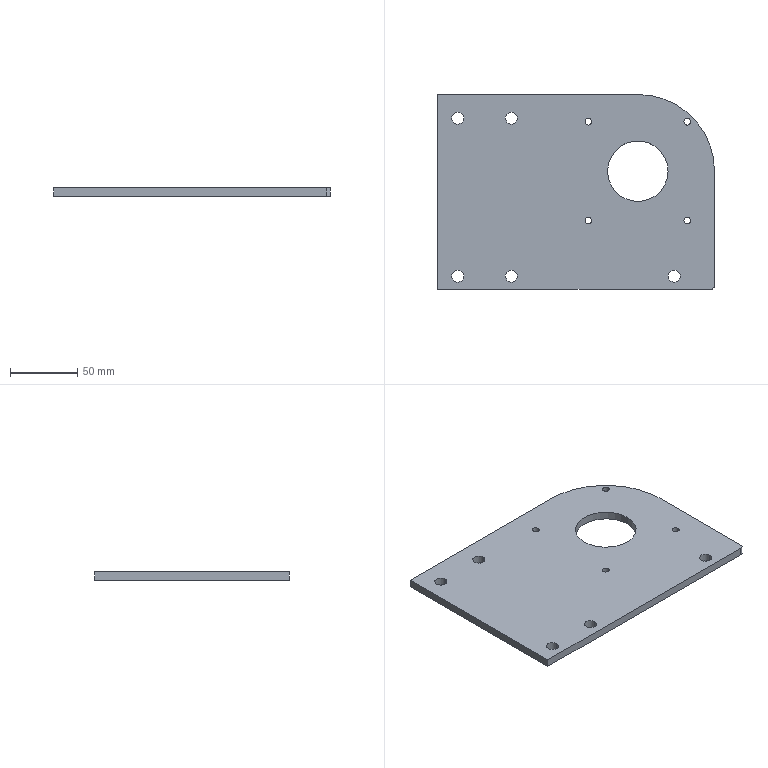Part | SolidWorks | features ICE 6, Fillet 5, HoleWzd 2, CirPattern 1, Extrusion 1 | 1 solid | 28 faces | box 206 x 145 x 6 mm | volume 163103 mm3 | cylinder 22 | plane 6 | commonest cylinder face diameters 9 x10 5 x8 45 x2 6 x1 114 x1
STEP:
#1=CARTESIAN_POINT('',(68.5,-62.5,0.));
#2=VERTEX_POINT('',#1);
#3=CARTESIAN_POINT('',(77.5,-62.5,0.));
#4=VERTEX_POINT('',#3);
#5=CARTESIAN_POINT('',(73.,-62.5,0.));
#6=DIRECTION('',(0.,0.,1.));
#7=DIRECTION('',(1.,0.,0.));
#8=AXIS2_PLACEMENT_3D('',#5,#6,#7);
#9=CIRCLE('',#8,4.5);
#10=EDGE_CURVE('',#2,#4,#9,.T.);
#11=ORIENTED_EDGE('',*,*,#10,.F.);
#12=CARTESIAN_POINT('',(68.5,-62.5,6.));
#13=VERTEX_POINT('',#12);
#14=CARTESIAN_POINT('',(68.5,-62.5,0.));
#15=DIRECTION('',(0.,0.,1.));
#16=VECTOR('',#15,1000.);
#17=LINE('',#14,#16);
#18=EDGE_CURVE('',#2,#13,#17,.T.);
#19=ORIENTED_EDGE('',*,*,#18,.T.);
#20=CARTESIAN_POINT('',(77.5,-62.5,6.));
#21=VERTEX_POINT('',#20);
#22=CARTESIAN_POINT('',(73.,-62.5,6.));
#23=DIRECTION('',(0.,0.,1.));
#24=DIRECTION('',(1.,0.,0.));
#25=AXIS2_PLACEMENT_3D('',#22,#23,#24);
#26=CIRCLE('',#25,4.5);
#27=EDGE_CURVE('',#13,#21,#26,.T.);
#28=ORIENTED_EDGE('',*,*,#27,.T.);
#29=CARTESIAN_POINT('',(77.5,-62.5,0.));
#30=DIRECTION('',(0.,0.,1.));
#31=VECTOR('',#30,1000.);
#32=LINE('',#29,#31);
#33=EDGE_CURVE('',#4,#21,#32,.T.);
#34=ORIENTED_EDGE('',*,*,#33,.F.);
#35=EDGE_LOOP('',(#11,#19,#28,#34));
#36=FACE_OUTER_BOUND('',#35,.T.);
#37=CARTESIAN_POINT('',(73.,-62.5,0.));
#38=DIRECTION('',(0.,0.,1.));
#39=DIRECTION('',(1.,0.,0.));
#40=AXIS2_PLACEMENT_3D('',#37,#38,#39);
#41=CYLINDRICAL_SURFACE('',#40,4.5);
#42=ADVANCED_FACE('',(#36),#41,.F.);
#43=CARTESIAN_POINT('',(80.27,52.27,0.));
#44=VERTEX_POINT('',#43);
#45=CARTESIAN_POINT('',(85.27,52.27,0.));
#46=VERTEX_POINT('',#45);
#47=CARTESIAN_POINT('',(82.77,52.27,0.));
#48=DIRECTION('',(0.,0.,1.));
#49=DIRECTION('',(1.,0.,0.));
#50=AXIS2_PLACEMENT_3D('',#47,#48,#49);
#51=CIRCLE('',#50,2.5);
#52=EDGE_CURVE('',#44,#46,#51,.T.);
#53=ORIENTED_EDGE('',*,*,#52,.F.);
#54=CARTESIAN_POINT('',(80.27,52.27,6.));
#55=VERTEX_POINT('',#54);
#56=CARTESIAN_POINT('',(80.27,52.27,6.));
#57=DIRECTION('',(0.,0.,1.));
#58=VECTOR('',#57,1000.);
#59=LINE('',#56,#58);
#60=EDGE_CURVE('',#44,#55,#59,.T.);
#61=ORIENTED_EDGE('',*,*,#60,.T.);
#62=CARTESIAN_POINT('',(85.27,52.27,6.));
#63=VERTEX_POINT('',#62);
#64=CARTESIAN_POINT('',(82.77,52.27,6.));
#65=DIRECTION('',(0.,0.,1.));
#66=DIRECTION('',(1.,0.,0.));
#67=AXIS2_PLACEMENT_3D('',#64,#65,#66);
#68=CIRCLE('',#67,2.5);
#69=EDGE_CURVE('',#55,#63,#68,.T.);
#70=ORIENTED_EDGE('',*,*,#69,.T.);
#71=CARTESIAN_POINT('',(85.27,52.27,6.));
#72=DIRECTION('',(0.,0.,1.));
#73=VECTOR('',#72,1000.);
#74=LINE('',#71,#73);
#75=EDGE_CURVE('',#46,#63,#74,.T.);
#76=ORIENTED_EDGE('',*,*,#75,.F.);
#77=EDGE_LOOP('',(#53,#61,#70,#76));
#78=FACE_OUTER_BOUND('',#77,.T.);
#79=CARTESIAN_POINT('',(82.77,52.27,6.));
#80=DIRECTION('',(0.,0.,1.));
#81=DIRECTION('',(1.,0.,0.));
#82=AXIS2_PLACEMENT_3D('',#79,#80,#81);
#83=CYLINDRICAL_SURFACE('',#82,2.5);
#84=ADVANCED_FACE('',(#78),#83,.F.);
#85=CARTESIAN_POINT('',(80.27,-21.27,0.));
#86=VERTEX_POINT('',#85);
#87=CARTESIAN_POINT('',(85.27,-21.27,0.));
#88=VERTEX_POINT('',#87);
#89=CARTESIAN_POINT('',(82.77,-21.27,0.));
#90=DIRECTION('',(0.,0.,1.));
#91=DIRECTION('',(1.,0.,0.));
#92=AXIS2_PLACEMENT_3D('',#89,#90,#91);
#93=CIRCLE('',#92,2.5);
#94=EDGE_CURVE('',#86,#88,#93,.T.);
#95=ORIENTED_EDGE('',*,*,#94,.F.);
#96=CARTESIAN_POINT('',(80.27,-21.27,6.));
#97=VERTEX_POINT('',#96);
#98=CARTESIAN_POINT('',(80.27,-21.27,6.));
#99=DIRECTION('',(0.,0.,1.));
#100=VECTOR('',#99,1000.);
#101=LINE('',#98,#100);
#102=EDGE_CURVE('',#86,#97,#101,.T.);
#103=ORIENTED_EDGE('',*,*,#102,.T.);
#104=CARTESIAN_POINT('',(85.27,-21.27,6.));
#105=VERTEX_POINT('',#104);
#106=CARTESIAN_POINT('',(82.77,-21.27,6.));
#107=DIRECTION('',(0.,0.,1.));
#108=DIRECTION('',(1.,0.,0.));
#109=AXIS2_PLACEMENT_3D('',#106,#107,#108);
#110=CIRCLE('',#109,2.5);
#111=EDGE_CURVE('',#97,#105,#110,.T.);
#112=ORIENTED_EDGE('',*,*,#111,.T.);
#113=CARTESIAN_POINT('',(85.27,-21.27,6.));
#114=DIRECTION('',(0.,0.,1.));
#115=VECTOR('',#114,1000.);
#116=LINE('',#113,#115);
#117=EDGE_CURVE('',#88,#105,#116,.T.);
#118=ORIENTED_EDGE('',*,*,#117,.F.);
#119=EDGE_LOOP('',(#95,#103,#112,#118));
#120=FACE_OUTER_BOUND('',#119,.T.);
#121=CARTESIAN_POINT('',(82.77,-21.27,6.));
#122=DIRECTION('',(0.,0.,1.));
#123=DIRECTION('',(1.,0.,0.));
#124=AXIS2_PLACEMENT_3D('',#121,#122,#123);
#125=CYLINDRICAL_SURFACE('',#124,2.5);
#126=ADVANCED_FACE('',(#120),#125,.F.);
#127=CARTESIAN_POINT('',(6.73,-21.27,0.));
#128=VERTEX_POINT('',#127);
#129=CARTESIAN_POINT('',(11.73,-21.27,0.));
#130=VERTEX_POINT('',#129);
#131=CARTESIAN_POINT('',(9.23,-21.27,0.));
#132=DIRECTION('',(0.,0.,1.));
#133=DIRECTION('',(1.,0.,0.));
#134=AXIS2_PLACEMENT_3D('',#131,#132,#133);
#135=CIRCLE('',#134,2.5);
#136=EDGE_CURVE('',#128,#130,#135,.T.);
#137=ORIENTED_EDGE('',*,*,#136,.F.);
#138=CARTESIAN_POINT('',(6.73,-21.27,6.));
#139=VERTEX_POINT('',#138);
#140=CARTESIAN_POINT('',(6.73,-21.27,6.));
#141=DIRECTION('',(0.,0.,1.));
#142=VECTOR('',#141,1000.);
#143=LINE('',#140,#142);
#144=EDGE_CURVE('',#128,#139,#143,.T.);
#145=ORIENTED_EDGE('',*,*,#144,.T.);
#146=CARTESIAN_POINT('',(11.73,-21.27,6.));
#147=VERTEX_POINT('',#146);
#148=CARTESIAN_POINT('',(9.23,-21.27,6.));
#149=DIRECTION('',(0.,0.,1.));
#150=DIRECTION('',(1.,0.,0.));
#151=AXIS2_PLACEMENT_3D('',#148,#149,#150);
#152=CIRCLE('',#151,2.5);
#153=EDGE_CURVE('',#139,#147,#152,.T.);
#154=ORIENTED_EDGE('',*,*,#153,.T.);
#155=CARTESIAN_POINT('',(11.73,-21.27,6.));
#156=DIRECTION('',(0.,0.,1.));
#157=VECTOR('',#156,1000.);
#158=LINE('',#155,#157);
#159=EDGE_CURVE('',#130,#147,#158,.T.);
#160=ORIENTED_EDGE('',*,*,#159,.F.);
#161=EDGE_LOOP('',(#137,#145,#154,#160));
#162=FACE_OUTER_BOUND('',#161,.T.);
#163=CARTESIAN_POINT('',(9.23,-21.27,6.));
#164=DIRECTION('',(0.,0.,1.));
#165=DIRECTION('',(1.,0.,0.));
#166=AXIS2_PLACEMENT_3D('',#163,#164,#165);
#167=CYLINDRICAL_SURFACE('',#166,2.5);
#168=ADVANCED_FACE('',(#162),#167,.F.);
#169=CARTESIAN_POINT('',(6.73,52.27,0.));
#170=VERTEX_POINT('',#169);
#171=CARTESIAN_POINT('',(11.73,52.27,0.));
#172=VERTEX_POINT('',#171);
#173=CARTESIAN_POINT('',(9.23,52.27,0.));
#174=DIRECTION('',(0.,0.,1.));
#175=DIRECTION('',(1.,0.,0.));
#176=AXIS2_PLACEMENT_3D('',#173,#174,#175);
#177=CIRCLE('',#176,2.5);
#178=EDGE_CURVE('',#170,#172,#177,.T.);
#179=ORIENTED_EDGE('',*,*,#178,.F.);
#180=CARTESIAN_POINT('',(6.73,52.27,6.));
#181=VERTEX_POINT('',#180);
#182=CARTESIAN_POINT('',(6.73,52.27,6.));
#183=DIRECTION('',(0.,0.,1.));
#184=VECTOR('',#183,1000.);
#185=LINE('',#182,#184);
#186=EDGE_CURVE('',#170,#181,#185,.T.);
#187=ORIENTED_EDGE('',*,*,#186,.T.);
#188=CARTESIAN_POINT('',(11.73,52.27,6.));
#189=VERTEX_POINT('',#188);
#190=CARTESIAN_POINT('',(9.23,52.27,6.));
#191=DIRECTION('',(0.,0.,1.));
#192=DIRECTION('',(1.,0.,0.));
#193=AXIS2_PLACEMENT_3D('',#190,#191,#192);
#194=CIRCLE('',#193,2.5);
#195=EDGE_CURVE('',#181,#189,#194,.T.);
#196=ORIENTED_EDGE('',*,*,#195,.T.);
#197=CARTESIAN_POINT('',(11.73,52.27,6.));
#198=DIRECTION('',(0.,0.,1.));
#199=VECTOR('',#198,1000.);
#200=LINE('',#197,#199);
#201=EDGE_CURVE('',#172,#189,#200,.T.);
#202=ORIENTED_EDGE('',*,*,#201,.F.);
#203=EDGE_LOOP('',(#179,#187,#196,#202));
#204=FACE_OUTER_BOUND('',#203,.T.);
#205=CARTESIAN_POINT('',(9.23,52.27,6.));
#206=DIRECTION('',(0.,0.,1.));
#207=DIRECTION('',(1.,0.,0.));
#208=AXIS2_PLACEMENT_3D('',#205,#206,#207);
#209=CYLINDRICAL_SURFACE('',#208,2.5);
#210=ADVANCED_FACE('',(#204),#209,.F.);
#211=CARTESIAN_POINT('',(23.5,15.5,0.));
#212=VERTEX_POINT('',#211);
#213=CARTESIAN_POINT('',(68.5,15.5,0.));
#214=VERTEX_POINT('',#213);
#215=CARTESIAN_POINT('',(46.,15.5,0.));
#216=DIRECTION('',(0.,0.,1.));
#217=DIRECTION('',(1.,0.,0.));
#218=AXIS2_PLACEMENT_3D('',#215,#216,#217);
#219=CIRCLE('',#218,22.5);
#220=EDGE_CURVE('',#212,#214,#219,.T.);
#221=ORIENTED_EDGE('',*,*,#220,.F.);
#222=CARTESIAN_POINT('',(23.5,15.5,6.));
#223=VERTEX_POINT('',#222);
#224=CARTESIAN_POINT('',(23.5,15.5,0.));
#225=DIRECTION('',(0.,0.,1.));
#226=VECTOR('',#225,1000.);
#227=LINE('',#224,#226);
#228=EDGE_CURVE('',#212,#223,#227,.T.);
#229=ORIENTED_EDGE('',*,*,#228,.T.);
#230=CARTESIAN_POINT('',(68.5,15.5,6.));
#231=VERTEX_POINT('',#230);
#232=CARTESIAN_POINT('',(46.,15.5,6.));
#233=DIRECTION('',(0.,0.,1.));
#234=DIRECTION('',(1.,0.,0.));
#235=AXIS2_PLACEMENT_3D('',#232,#233,#234);
#236=CIRCLE('',#235,22.5);
#237=EDGE_CURVE('',#223,#231,#236,.T.);
#238=ORIENTED_EDGE('',*,*,#237,.T.);
#239=CARTESIAN_POINT('',(68.5,15.5,0.));
#240=DIRECTION('',(0.,0.,1.));
#241=VECTOR('',#240,1000.);
#242=LINE('',#239,#241);
#243=EDGE_CURVE('',#214,#231,#242,.T.);
#244=ORIENTED_EDGE('',*,*,#243,.F.);
#245=EDGE_LOOP('',(#221,#229,#238,#244));
#246=FACE_OUTER_BOUND('',#245,.T.);
#247=CARTESIAN_POINT('',(46.,15.5,0.));
#248=DIRECTION('',(0.,0.,1.));
#249=DIRECTION('',(1.,0.,0.));
#250=AXIS2_PLACEMENT_3D('',#247,#248,#249);
#251=CYLINDRICAL_SURFACE('',#250,22.5);
#252=ADVANCED_FACE('',(#246),#251,.F.);
#253=CARTESIAN_POINT('',(-52.5,-62.5,0.));
#254=VERTEX_POINT('',#253);
#255=CARTESIAN_POINT('',(-43.5,-62.5,0.));
#256=VERTEX_POINT('',#255);
#257=CARTESIAN_POINT('',(-48.,-62.5,0.));
#258=DIRECTION('',(0.,0.,1.));
#259=DIRECTION('',(1.,0.,0.));
#260=AXIS2_PLACEMENT_3D('',#257,#258,#259);
#261=CIRCLE('',#260,4.5);
#262=EDGE_CURVE('',#254,#256,#261,.T.);
#263=ORIENTED_EDGE('',*,*,#262,.F.);
#264=CARTESIAN_POINT('',(-52.5,-62.5,6.));
#265=VERTEX_POINT('',#264);
#266=CARTESIAN_POINT('',(-52.5,-62.5,0.));
#267=DIRECTION('',(0.,0.,1.));
#268=VECTOR('',#267,1000.);
#269=LINE('',#266,#268);
#270=EDGE_CURVE('',#254,#265,#269,.T.);
#271=ORIENTED_EDGE('',*,*,#270,.T.);
#272=CARTESIAN_POINT('',(-43.5,-62.5,6.));
#273=VERTEX_POINT('',#272);
#274=CARTESIAN_POINT('',(-48.,-62.5,6.));
#275=DIRECTION('',(0.,0.,1.));
#276=DIRECTION('',(1.,0.,0.));
#277=AXIS2_PLACEMENT_3D('',#274,#275,#276);
#278=CIRCLE('',#277,4.5);
#279=EDGE_CURVE('',#265,#273,#278,.T.);
#280=ORIENTED_EDGE('',*,*,#279,.T.);
#281=CARTESIAN_POINT('',(-43.5,-62.5,0.));
#282=DIRECTION('',(0.,0.,1.));
#283=VECTOR('',#282,1000.);
#284=LINE('',#281,#283);
#285=EDGE_CURVE('',#256,#273,#284,.T.);
#286=ORIENTED_EDGE('',*,*,#285,.F.);
#287=EDGE_LOOP('',(#263,#271,#280,#286));
#288=FACE_OUTER_BOUND('',#287,.T.);
#289=CARTESIAN_POINT('',(-48.,-62.5,0.));
#290=DIRECTION('',(0.,0.,1.));
#291=DIRECTION('',(1.,0.,0.));
#292=AXIS2_PLACEMENT_3D('',#289,#290,#291);
#293=CYLINDRICAL_SURFACE('',#292,4.5);
#294=ADVANCED_FACE('',(#288),#293,.F.);
#295=CARTESIAN_POINT('',(-92.5,-62.5,0.));
#296=VERTEX_POINT('',#295);
#297=CARTESIAN_POINT('',(-83.5,-62.5,0.));
#298=VERTEX_POINT('',#297);
#299=CARTESIAN_POINT('',(-88.,-62.5,0.));
#300=DIRECTION('',(0.,0.,1.));
#301=DIRECTION('',(1.,0.,0.));
#302=AXIS2_PLACEMENT_3D('',#299,#300,#301);
#303=CIRCLE('',#302,4.5);
#304=EDGE_CURVE('',#296,#298,#303,.T.);
#305=ORIENTED_EDGE('',*,*,#304,.F.);
#306=CARTESIAN_POINT('',(-92.5,-62.5,6.));
#307=VERTEX_POINT('',#306);
#308=CARTESIAN_POINT('',(-92.5,-62.5,0.));
#309=DIRECTION('',(0.,0.,1.));
#310=VECTOR('',#309,1000.);
#311=LINE('',#308,#310);
#312=EDGE_CURVE('',#296,#307,#311,.T.);
#313=ORIENTED_EDGE('',*,*,#312,.T.);
#314=CARTESIAN_POINT('',(-83.5,-62.5,6.));
#315=VERTEX_POINT('',#314);
#316=CARTESIAN_POINT('',(-88.,-62.5,6.));
#317=DIRECTION('',(0.,0.,1.));
#318=DIRECTION('',(1.,0.,0.));
#319=AXIS2_PLACEMENT_3D('',#316,#317,#318);
#320=CIRCLE('',#319,4.5);
#321=EDGE_CURVE('',#307,#315,#320,.T.);
#322=ORIENTED_EDGE('',*,*,#321,.T.);
#323=CARTESIAN_POINT('',(-83.5,-62.5,0.));
#324=DIRECTION('',(0.,0.,1.));
#325=VECTOR('',#324,1000.);
#326=LINE('',#323,#325);
#327=EDGE_CURVE('',#298,#315,#326,.T.);
#328=ORIENTED_EDGE('',*,*,#327,.F.);
#329=EDGE_LOOP('',(#305,#313,#322,#328));
#330=FACE_OUTER_BOUND('',#329,.T.);
#331=CARTESIAN_POINT('',(-88.,-62.5,0.));
#332=DIRECTION('',(0.,0.,1.));
#333=DIRECTION('',(1.,0.,0.));
#334=AXIS2_PLACEMENT_3D('',#331,#332,#333);
#335=CYLINDRICAL_SURFACE('',#334,4.5);
#336=ADVANCED_FACE('',(#330),#335,.F.);
#337=CARTESIAN_POINT('',(-52.5,55.,0.));
#338=VERTEX_POINT('',#337);
#339=CARTESIAN_POINT('',(-43.5,55.,0.));
#340=VERTEX_POINT('',#339);
#341=CARTESIAN_POINT('',(-48.,55.,0.));
#342=DIRECTION('',(0.,0.,1.));
#343=DIRECTION('',(1.,0.,0.));
#344=AXIS2_PLACEMENT_3D('',#341,#342,#343);
#345=CIRCLE('',#344,4.5);
#346=EDGE_CURVE('',#338,#340,#345,.T.);
#347=ORIENTED_EDGE('',*,*,#346,.F.);
#348=CARTESIAN_POINT('',(-52.5,55.,6.));
#349=VERTEX_POINT('',#348);
#350=CARTESIAN_POINT('',(-52.5,55.,0.));
#351=DIRECTION('',(0.,0.,1.));
#352=VECTOR('',#351,1000.);
#353=LINE('',#350,#352);
#354=EDGE_CURVE('',#338,#349,#353,.T.);
#355=ORIENTED_EDGE('',*,*,#354,.T.);
#356=CARTESIAN_POINT('',(-43.5,55.,6.));
#357=VERTEX_POINT('',#356);
#358=CARTESIAN_POINT('',(-48.,55.,6.));
#359=DIRECTION('',(0.,0.,1.));
#360=DIRECTION('',(1.,0.,0.));
#361=AXIS2_PLACEMENT_3D('',#358,#359,#360);
#362=CIRCLE('',#361,4.5);
#363=EDGE_CURVE('',#349,#357,#362,.T.);
#364=ORIENTED_EDGE('',*,*,#363,.T.);
#365=CARTESIAN_POINT('',(-43.5,55.,0.));
#366=DIRECTION('',(0.,0.,1.));
#367=VECTOR('',#366,1000.);
#368=LINE('',#365,#367);
#369=EDGE_CURVE('',#340,#357,#368,.T.);
#370=ORIENTED_EDGE('',*,*,#369,.F.);
#371=EDGE_LOOP('',(#347,#355,#364,#370));
#372=FACE_OUTER_BOUND('',#371,.T.);
#373=CARTESIAN_POINT('',(-48.,55.,0.));
#374=DIRECTION('',(0.,0.,1.));
#375=DIRECTION('',(1.,0.,0.));
#376=AXIS2_PLACEMENT_3D('',#373,#374,#375);
#377=CYLINDRICAL_SURFACE('',#376,4.5);
#378=ADVANCED_FACE('',(#372),#377,.F.);
#379=CARTESIAN_POINT('',(-92.5,55.,0.));
#380=VERTEX_POINT('',#379);
#381=CARTESIAN_POINT('',(-83.5,55.,0.));
#382=VERTEX_POINT('',#381);
#383=CARTESIAN_POINT('',(-88.,55.,0.));
#384=DIRECTION('',(0.,0.,1.));
#385=DIRECTION('',(1.,0.,0.));
#386=AXIS2_PLACEMENT_3D('',#383,#384,#385);
#387=CIRCLE('',#386,4.5);
#388=EDGE_CURVE('',#380,#382,#387,.T.);
#389=ORIENTED_EDGE('',*,*,#388,.F.);
#390=CARTESIAN_POINT('',(-92.5,55.,6.));
#391=VERTEX_POINT('',#390);
#392=CARTESIAN_POINT('',(-92.5,55.,0.));
#393=DIRECTION('',(0.,0.,1.));
#394=VECTOR('',#393,1000.);
#395=LINE('',#392,#394);
#396=EDGE_CURVE('',#380,#391,#395,.T.);
#397=ORIENTED_EDGE('',*,*,#396,.T.);
#398=CARTESIAN_POINT('',(-83.5,55.,6.));
#399=VERTEX_POINT('',#398);
#400=CARTESIAN_POINT('',(-88.,55.,6.));
#401=DIRECTION('',(0.,0.,1.));
#402=DIRECTION('',(1.,0.,0.));
#403=AXIS2_PLACEMENT_3D('',#400,#401,#402);
#404=CIRCLE('',#403,4.5);
#405=EDGE_CURVE('',#391,#399,#404,.T.);
#406=ORIENTED_EDGE('',*,*,#405,.T.);
#407=CARTESIAN_POINT('',(-83.5,55.,0.));
#408=DIRECTION('',(0.,0.,1.));
#409=VECTOR('',#408,1000.);
#410=LINE('',#407,#409);
#411=EDGE_CURVE('',#382,#399,#410,.T.);
#412=ORIENTED_EDGE('',*,*,#411,.F.);
#413=EDGE_LOOP('',(#389,#397,#406,#412));
#414=FACE_OUTER_BOUND('',#413,.T.);
#415=CARTESIAN_POINT('',(-88.,55.,0.));
#416=DIRECTION('',(0.,0.,1.));
#417=DIRECTION('',(1.,0.,0.));
#418=AXIS2_PLACEMENT_3D('',#415,#416,#417);
#419=CYLINDRICAL_SURFACE('',#418,4.5);
#420=ADVANCED_FACE('',(#414),#419,.F.);
#421=CARTESIAN_POINT('',(-103.,72.5,0.));
#422=VERTEX_POINT('',#421);
#423=CARTESIAN_POINT('',(-103.,-72.5,0.));
#424=VERTEX_POINT('',#423);
#425=CARTESIAN_POINT('',(-103.,72.5,0.));
#426=DIRECTION('',(0.,-1.,0.));
#427=VECTOR('',#426,1000.);
#428=LINE('',#425,#427);
#429=EDGE_CURVE('',#422,#424,#428,.T.);
#430=ORIENTED_EDGE('',*,*,#429,.T.);
#431=CARTESIAN_POINT('',(-103.,-72.5,6.));
#432=VERTEX_POINT('',#431);
#433=CARTESIAN_POINT('',(-103.,-72.5,6.));
#434=DIRECTION('',(0.,0.,-1.));
#435=VECTOR('',#434,1000.);
#436=LINE('',#433,#435);
#437=EDGE_CURVE('',#432,#424,#436,.T.);
#438=ORIENTED_EDGE('',*,*,#437,.F.);
#439=CARTESIAN_POINT('',(-103.,72.5,6.));
#440=VERTEX_POINT('',#439);
#441=CARTESIAN_POINT('',(-103.,72.5,6.));
#442=DIRECTION('',(0.,-1.,0.));
#443=VECTOR('',#442,1000.);
#444=LINE('',#441,#443);
#445=EDGE_CURVE('',#440,#432,#444,.T.);
#446=ORIENTED_EDGE('',*,*,#445,.F.);
#447=CARTESIAN_POINT('',(-103.,72.5,6.));
#448=DIRECTION('',(0.,0.,-1.));
#449=VECTOR('',#448,1000.);
#450=LINE('',#447,#449);
#451=EDGE_CURVE('',#440,#422,#450,.T.);
#452=ORIENTED_EDGE('',*,*,#451,.T.);
#453=EDGE_LOOP('',(#430,#438,#446,#452));
#454=FACE_OUTER_BOUND('',#453,.T.);
#455=CARTESIAN_POINT('',(-103.,72.5,6.));
#456=DIRECTION('',(1.,0.,0.));
#457=DIRECTION('',(0.,0.,-1.));
#458=AXIS2_PLACEMENT_3D('',#455,#456,#457);
#459=PLANE('',#458);
#460=ADVANCED_FACE('',(#454),#459,.F.);
#461=CARTESIAN_POINT('',(100.,-72.5,0.));
#462=VERTEX_POINT('',#461);
#463=CARTESIAN_POINT('',(-103.,-72.5,0.));
#464=DIRECTION('',(1.,0.,0.));
#465=VECTOR('',#464,1000.);
#466=LINE('',#463,#465);
#467=EDGE_CURVE('',#424,#462,#466,.T.);
#468=ORIENTED_EDGE('',*,*,#467,.T.);
#469=CARTESIAN_POINT('',(100.,-72.5,6.));
#470=VERTEX_POINT('',#469);
#471=CARTESIAN_POINT('',(100.,-72.5,6.));
#472=DIRECTION('',(0.,0.,1.));
#473=VECTOR('',#472,1000.);
#474=LINE('',#471,#473);
#475=EDGE_CURVE('',#462,#470,#474,.T.);
#476=ORIENTED_EDGE('',*,*,#475,.T.);
#477=CARTESIAN_POINT('',(-103.,-72.5,6.));
#478=DIRECTION('',(1.,0.,0.));
#479=VECTOR('',#478,1000.);
#480=LINE('',#477,#479);
#481=EDGE_CURVE('',#432,#470,#480,.T.);
#482=ORIENTED_EDGE('',*,*,#481,.F.);
#483=ORIENTED_EDGE('',*,*,#437,.T.);
#484=EDGE_LOOP('',(#468,#476,#482,#483));
#485=FACE_OUTER_BOUND('',#484,.T.);
#486=CARTESIAN_POINT('',(-103.,-72.5,6.));
#487=DIRECTION('',(0.,1.,0.));
#488=DIRECTION('',(0.,0.,1.));
#489=AXIS2_PLACEMENT_3D('',#486,#487,#488);
#490=PLANE('',#489);
#491=ADVANCED_FACE('',(#485),#490,.F.);
#492=CARTESIAN_POINT('',(103.,-69.5,6.));
#493=VERTEX_POINT('',#492);
#494=CARTESIAN_POINT('',(103.,15.5,6.));
#495=VERTEX_POINT('',#494);
#496=CARTESIAN_POINT('',(103.,72.5,6.));
#497=DIRECTION('',(0.,1.,0.));
#498=VECTOR('',#497,1000.);
#499=LINE('',#496,#498);
#500=EDGE_CURVE('',#493,#495,#499,.T.);
#501=ORIENTED_EDGE('',*,*,#500,.F.);
#502=CARTESIAN_POINT('',(103.,-69.5,0.));
#503=VERTEX_POINT('',#502);
#504=CARTESIAN_POINT('',(103.,-69.5,6.));
#505=DIRECTION('',(0.,0.,-1.));
#506=VECTOR('',#505,1000.);
#507=LINE('',#504,#506);
#508=EDGE_CURVE('',#493,#503,#507,.T.);
#509=ORIENTED_EDGE('',*,*,#508,.T.);
#510=CARTESIAN_POINT('',(103.,15.5,0.));
#511=VERTEX_POINT('',#510);
#512=CARTESIAN_POINT('',(103.,72.5,0.));
#513=DIRECTION('',(0.,1.,0.));
#514=VECTOR('',#513,1000.);
#515=LINE('',#512,#514);
#516=EDGE_CURVE('',#503,#511,#515,.T.);
#517=ORIENTED_EDGE('',*,*,#516,.T.);
#518=CARTESIAN_POINT('',(103.,15.5,6.));
#519=DIRECTION('',(0.,0.,1.));
#520=VECTOR('',#519,1000.);
#521=LINE('',#518,#520);
#522=EDGE_CURVE('',#511,#495,#521,.T.);
#523=ORIENTED_EDGE('',*,*,#522,.T.);
#524=EDGE_LOOP('',(#501,#509,#517,#523));
#525=FACE_OUTER_BOUND('',#524,.T.);
#526=CARTESIAN_POINT('',(103.,72.5,6.));
#527=DIRECTION('',(-1.,0.,0.));
#528=DIRECTION('',(0.,0.,1.));
#529=AXIS2_PLACEMENT_3D('',#526,#527,#528);
#530=PLANE('',#529);
#531=ADVANCED_FACE('',(#525),#530,.F.);
#532=CARTESIAN_POINT('',(46.,72.5,6.));
#533=VERTEX_POINT('',#532);
#534=CARTESIAN_POINT('',(-103.,72.5,6.));
#535=DIRECTION('',(-1.,0.,0.));
#536=VECTOR('',#535,1000.);
#537=LINE('',#534,#536);
#538=EDGE_CURVE('',#533,#440,#537,.T.);
#539=ORIENTED_EDGE('',*,*,#538,.F.);
#540=CARTESIAN_POINT('',(46.,72.5,0.));
#541=VERTEX_POINT('',#540);
#542=CARTESIAN_POINT('',(46.,72.5,6.));
#543=DIRECTION('',(0.,0.,-1.));
#544=VECTOR('',#543,1000.);
#545=LINE('',#542,#544);
#546=EDGE_CURVE('',#533,#541,#545,.T.);
#547=ORIENTED_EDGE('',*,*,#546,.T.);
#548=CARTESIAN_POINT('',(-103.,72.5,0.));
#549=DIRECTION('',(-1.,0.,0.));
#550=VECTOR('',#549,1000.);
#551=LINE('',#548,#550);
#552=EDGE_CURVE('',#541,#422,#551,.T.);
#553=ORIENTED_EDGE('',*,*,#552,.T.);
#554=ORIENTED_EDGE('',*,*,#451,.F.);
#555=EDGE_LOOP('',(#539,#547,#553,#554));
#556=FACE_OUTER_BOUND('',#555,.T.);
#557=CARTESIAN_POINT('',(-103.,72.5,6.));
#558=DIRECTION('',(0.,-1.,0.));
#559=DIRECTION('',(0.,0.,-1.));
#560=AXIS2_PLACEMENT_3D('',#557,#558,#559);
#561=PLANE('',#560);
#562=ADVANCED_FACE('',(#556),#561,.F.);
#563=CARTESIAN_POINT('',(73.,-62.5,6.));
#564=DIRECTION('',(0.,0.,1.));
#565=DIRECTION('',(1.,0.,0.));
#566=AXIS2_PLACEMENT_3D('',#563,#564,#565);
#567=CIRCLE('',#566,4.5);
#568=EDGE_CURVE('',#21,#13,#567,.T.);
#569=ORIENTED_EDGE('',*,*,#568,.F.);
#570=ORIENTED_EDGE('',*,*,#27,.F.);
#571=EDGE_LOOP('',(#569,#570));
#572=FACE_BOUND('',#571,.T.);
#573=CARTESIAN_POINT('',(82.77,52.27,6.));
#574=DIRECTION('',(0.,0.,1.));
#575=DIRECTION('',(1.,0.,0.));
#576=AXIS2_PLACEMENT_3D('',#573,#574,#575);
#577=CIRCLE('',#576,2.5);
#578=EDGE_CURVE('',#63,#55,#577,.T.);
#579=ORIENTED_EDGE('',*,*,#578,.F.);
#580=ORIENTED_EDGE('',*,*,#69,.F.);
#581=EDGE_LOOP('',(#579,#580));
#582=FACE_BOUND('',#581,.T.);
#583=CARTESIAN_POINT('',(82.77,-21.27,6.));
#584=DIRECTION('',(0.,0.,1.));
#585=DIRECTION('',(1.,0.,0.));
#586=AXIS2_PLACEMENT_3D('',#583,#584,#585);
#587=CIRCLE('',#586,2.5);
#588=EDGE_CURVE('',#105,#97,#587,.T.);
#589=ORIENTED_EDGE('',*,*,#588,.F.);
#590=ORIENTED_EDGE('',*,*,#111,.F.);
#591=EDGE_LOOP('',(#589,#590));
#592=FACE_BOUND('',#591,.T.);
#593=CARTESIAN_POINT('',(9.23,-21.27,6.));
#594=DIRECTION('',(0.,0.,1.));
#595=DIRECTION('',(1.,0.,0.));
#596=AXIS2_PLACEMENT_3D('',#593,#594,#595);
#597=CIRCLE('',#596,2.5);
#598=EDGE_CURVE('',#147,#139,#597,.T.);
#599=ORIENTED_EDGE('',*,*,#598,.F.);
#600=ORIENTED_EDGE('',*,*,#153,.F.);
#601=EDGE_LOOP('',(#599,#600));
#602=FACE_BOUND('',#601,.T.);
#603=CARTESIAN_POINT('',(9.23,52.27,6.));
#604=DIRECTION('',(0.,0.,1.));
#605=DIRECTION('',(1.,0.,0.));
#606=AXIS2_PLACEMENT_3D('',#603,#604,#605);
#607=CIRCLE('',#606,2.5);
#608=EDGE_CURVE('',#189,#181,#607,.T.);
#609=ORIENTED_EDGE('',*,*,#608,.F.);
#610=ORIENTED_EDGE('',*,*,#195,.F.);
#611=EDGE_LOOP('',(#609,#610));
#612=FACE_BOUND('',#611,.T.);
#613=CARTESIAN_POINT('',(46.,15.5,6.));
#614=DIRECTION('',(0.,0.,1.));
#615=DIRECTION('',(1.,0.,0.));
#616=AXIS2_PLACEMENT_3D('',#613,#614,#615);
#617=CIRCLE('',#616,22.5);
#618=EDGE_CURVE('',#231,#223,#617,.T.);
#619=ORIENTED_EDGE('',*,*,#618,.F.);
#620=ORIENTED_EDGE('',*,*,#237,.F.);
#621=EDGE_LOOP('',(#619,#620));
#622=FACE_BOUND('',#621,.T.);
#623=CARTESIAN_POINT('',(-48.,-62.5,6.));
#624=DIRECTION('',(0.,0.,1.));
#625=DIRECTION('',(1.,0.,0.));
#626=AXIS2_PLACEMENT_3D('',#623,#624,#625);
#627=CIRCLE('',#626,4.5);
#628=EDGE_CURVE('',#273,#265,#627,.T.);
#629=ORIENTED_EDGE('',*,*,#628,.F.);
#630=ORIENTED_EDGE('',*,*,#279,.F.);
#631=EDGE_LOOP('',(#629,#630));
#632=FACE_BOUND('',#631,.T.);
#633=CARTESIAN_POINT('',(-88.,-62.5,6.));
#634=DIRECTION('',(0.,0.,1.));
#635=DIRECTION('',(1.,0.,0.));
#636=AXIS2_PLACEMENT_3D('',#633,#634,#635);
#637=CIRCLE('',#636,4.5);
#638=EDGE_CURVE('',#315,#307,#637,.T.);
#639=ORIENTED_EDGE('',*,*,#638,.F.);
#640=ORIENTED_EDGE('',*,*,#321,.F.);
#641=EDGE_LOOP('',(#639,#640));
#642=FACE_BOUND('',#641,.T.);
#643=CARTESIAN_POINT('',(-48.,55.,6.));
#644=DIRECTION('',(0.,0.,1.));
#645=DIRECTION('',(1.,0.,0.));
#646=AXIS2_PLACEMENT_3D('',#643,#644,#645);
#647=CIRCLE('',#646,4.5);
#648=EDGE_CURVE('',#357,#349,#647,.T.);
#649=ORIENTED_EDGE('',*,*,#648,.F.);
#650=ORIENTED_EDGE('',*,*,#363,.F.);
#651=EDGE_LOOP('',(#649,#650));
#652=FACE_BOUND('',#651,.T.);
#653=CARTESIAN_POINT('',(-88.,55.,6.));
#654=DIRECTION('',(0.,0.,1.));
#655=DIRECTION('',(1.,0.,0.));
#656=AXIS2_PLACEMENT_3D('',#653,#654,#655);
#657=CIRCLE('',#656,4.5);
#658=EDGE_CURVE('',#399,#391,#657,.T.);
#659=ORIENTED_EDGE('',*,*,#658,.F.);
#660=ORIENTED_EDGE('',*,*,#405,.F.);
#661=EDGE_LOOP('',(#659,#660));
#662=FACE_BOUND('',#661,.T.);
#663=ORIENTED_EDGE('',*,*,#481,.T.);
#664=CARTESIAN_POINT('',(100.,-69.5,6.));
#665=DIRECTION('',(0.,0.,1.));
#666=DIRECTION('',(1.,0.,0.));
#667=AXIS2_PLACEMENT_3D('',#664,#665,#666);
#668=CIRCLE('',#667,3.);
#669=EDGE_CURVE('',#470,#493,#668,.T.);
#670=ORIENTED_EDGE('',*,*,#669,.T.);
#671=ORIENTED_EDGE('',*,*,#500,.T.);
#672=CARTESIAN_POINT('',(46.,15.5,6.));
#673=DIRECTION('',(0.,0.,1.));
#674=DIRECTION('',(1.,0.,0.));
#675=AXIS2_PLACEMENT_3D('',#672,#673,#674);
#676=CIRCLE('',#675,57.);
#677=EDGE_CURVE('',#495,#533,#676,.T.);
#678=ORIENTED_EDGE('',*,*,#677,.T.);
#679=ORIENTED_EDGE('',*,*,#538,.T.);
#680=ORIENTED_EDGE('',*,*,#445,.T.);
#681=EDGE_LOOP('',(#663,#670,#671,#678,#679,#680));
#682=FACE_OUTER_BOUND('',#681,.T.);
#683=CARTESIAN_POINT('',(0.,0.,6.));
#684=DIRECTION('',(0.,0.,1.));
#685=DIRECTION('',(1.,0.,0.));
#686=AXIS2_PLACEMENT_3D('',#683,#684,#685);
#687=PLANE('',#686);
#688=ADVANCED_FACE('',(#572,#582,#592,#602,#612,#622,#632,#642,#652,#662,#682),#687,.T.);
#689=CARTESIAN_POINT('',(73.,-62.5,0.));
#690=DIRECTION('',(0.,0.,1.));
#691=DIRECTION('',(1.,0.,0.));
#692=AXIS2_PLACEMENT_3D('',#689,#690,#691);
#693=CIRCLE('',#692,4.5);
#694=EDGE_CURVE('',#4,#2,#693,.T.);
#695=ORIENTED_EDGE('',*,*,#694,.T.);
#696=ORIENTED_EDGE('',*,*,#10,.T.);
#697=EDGE_LOOP('',(#695,#696));
#698=FACE_BOUND('',#697,.T.);
#699=CARTESIAN_POINT('',(82.77,52.27,0.));
#700=DIRECTION('',(0.,0.,1.));
#701=DIRECTION('',(1.,0.,0.));
#702=AXIS2_PLACEMENT_3D('',#699,#700,#701);
#703=CIRCLE('',#702,2.5);
#704=EDGE_CURVE('',#46,#44,#703,.T.);
#705=ORIENTED_EDGE('',*,*,#704,.T.);
#706=ORIENTED_EDGE('',*,*,#52,.T.);
#707=EDGE_LOOP('',(#705,#706));
#708=FACE_BOUND('',#707,.T.);
#709=CARTESIAN_POINT('',(82.77,-21.27,0.));
#710=DIRECTION('',(0.,0.,1.));
#711=DIRECTION('',(1.,0.,0.));
#712=AXIS2_PLACEMENT_3D('',#709,#710,#711);
#713=CIRCLE('',#712,2.5);
#714=EDGE_CURVE('',#88,#86,#713,.T.);
#715=ORIENTED_EDGE('',*,*,#714,.T.);
#716=ORIENTED_EDGE('',*,*,#94,.T.);
#717=EDGE_LOOP('',(#715,#716));
#718=FACE_BOUND('',#717,.T.);
#719=CARTESIAN_POINT('',(9.23,-21.27,0.));
#720=DIRECTION('',(0.,0.,1.));
#721=DIRECTION('',(1.,0.,0.));
#722=AXIS2_PLACEMENT_3D('',#719,#720,#721);
#723=CIRCLE('',#722,2.5);
#724=EDGE_CURVE('',#130,#128,#723,.T.);
#725=ORIENTED_EDGE('',*,*,#724,.T.);
#726=ORIENTED_EDGE('',*,*,#136,.T.);
#727=EDGE_LOOP('',(#725,#726));
#728=FACE_BOUND('',#727,.T.);
#729=CARTESIAN_POINT('',(9.23,52.27,0.));
#730=DIRECTION('',(0.,0.,1.));
#731=DIRECTION('',(1.,0.,0.));
#732=AXIS2_PLACEMENT_3D('',#729,#730,#731);
#733=CIRCLE('',#732,2.5);
#734=EDGE_CURVE('',#172,#170,#733,.T.);
#735=ORIENTED_EDGE('',*,*,#734,.T.);
#736=ORIENTED_EDGE('',*,*,#178,.T.);
#737=EDGE_LOOP('',(#735,#736));
#738=FACE_BOUND('',#737,.T.);
#739=CARTESIAN_POINT('',(46.,15.5,0.));
#740=DIRECTION('',(0.,0.,1.));
#741=DIRECTION('',(1.,0.,0.));
#742=AXIS2_PLACEMENT_3D('',#739,#740,#741);
#743=CIRCLE('',#742,22.5);
#744=EDGE_CURVE('',#214,#212,#743,.T.);
#745=ORIENTED_EDGE('',*,*,#744,.T.);
#746=ORIENTED_EDGE('',*,*,#220,.T.);
#747=EDGE_LOOP('',(#745,#746));
#748=FACE_BOUND('',#747,.T.);
#749=CARTESIAN_POINT('',(-48.,-62.5,0.));
#750=DIRECTION('',(0.,0.,1.));
#751=DIRECTION('',(1.,0.,0.));
#752=AXIS2_PLACEMENT_3D('',#749,#750,#751);
#753=CIRCLE('',#752,4.5);
#754=EDGE_CURVE('',#256,#254,#753,.T.);
#755=ORIENTED_EDGE('',*,*,#754,.T.);
#756=ORIENTED_EDGE('',*,*,#262,.T.);
#757=EDGE_LOOP('',(#755,#756));
#758=FACE_BOUND('',#757,.T.);
#759=CARTESIAN_POINT('',(-88.,-62.5,0.));
#760=DIRECTION('',(0.,0.,1.));
#761=DIRECTION('',(1.,0.,0.));
#762=AXIS2_PLACEMENT_3D('',#759,#760,#761);
#763=CIRCLE('',#762,4.5);
#764=EDGE_CURVE('',#298,#296,#763,.T.);
#765=ORIENTED_EDGE('',*,*,#764,.T.);
#766=ORIENTED_EDGE('',*,*,#304,.T.);
#767=EDGE_LOOP('',(#765,#766));
#768=FACE_BOUND('',#767,.T.);
#769=CARTESIAN_POINT('',(-48.,55.,0.));
#770=DIRECTION('',(0.,0.,1.));
#771=DIRECTION('',(1.,0.,0.));
#772=AXIS2_PLACEMENT_3D('',#769,#770,#771);
#773=CIRCLE('',#772,4.5);
#774=EDGE_CURVE('',#340,#338,#773,.T.);
#775=ORIENTED_EDGE('',*,*,#774,.T.);
#776=ORIENTED_EDGE('',*,*,#346,.T.);
#777=EDGE_LOOP('',(#775,#776));
#778=FACE_BOUND('',#777,.T.);
#779=CARTESIAN_POINT('',(-88.,55.,0.));
#780=DIRECTION('',(0.,0.,1.));
#781=DIRECTION('',(1.,0.,0.));
#782=AXIS2_PLACEMENT_3D('',#779,#780,#781);
#783=CIRCLE('',#782,4.5);
#784=EDGE_CURVE('',#382,#380,#783,.T.);
#785=ORIENTED_EDGE('',*,*,#784,.T.);
#786=ORIENTED_EDGE('',*,*,#388,.T.);
#787=EDGE_LOOP('',(#785,#786));
#788=FACE_BOUND('',#787,.T.);
#789=ORIENTED_EDGE('',*,*,#516,.F.);
#790=CARTESIAN_POINT('',(100.,-69.5,0.));
#791=DIRECTION('',(0.,0.,-1.));
#792=DIRECTION('',(1.,0.,0.));
#793=AXIS2_PLACEMENT_3D('',#790,#791,#792);
#794=CIRCLE('',#793,3.);
#795=EDGE_CURVE('',#503,#462,#794,.T.);
#796=ORIENTED_EDGE('',*,*,#795,.T.);
#797=ORIENTED_EDGE('',*,*,#467,.F.);
#798=ORIENTED_EDGE('',*,*,#429,.F.);
#799=ORIENTED_EDGE('',*,*,#552,.F.);
#800=CARTESIAN_POINT('',(46.,15.5,0.));
#801=DIRECTION('',(0.,0.,-1.));
#802=DIRECTION('',(1.,0.,0.));
#803=AXIS2_PLACEMENT_3D('',#800,#801,#802);
#804=CIRCLE('',#803,57.);
#805=EDGE_CURVE('',#541,#511,#804,.T.);
#806=ORIENTED_EDGE('',*,*,#805,.T.);
#807=EDGE_LOOP('',(#789,#796,#797,#798,#799,#806));
#808=FACE_OUTER_BOUND('',#807,.T.);
#809=CARTESIAN_POINT('',(0.,0.,0.));
#810=DIRECTION('',(0.,0.,1.));
#811=DIRECTION('',(1.,0.,0.));
#812=AXIS2_PLACEMENT_3D('',#809,#810,#811);
#813=PLANE('',#812);
#814=ADVANCED_FACE('',(#698,#708,#718,#728,#738,#748,#758,#768,#778,#788,#808),#813,.F.);
#815=ORIENTED_EDGE('',*,*,#396,.F.);
#816=ORIENTED_EDGE('',*,*,#784,.F.);
#817=ORIENTED_EDGE('',*,*,#411,.T.);
#818=ORIENTED_EDGE('',*,*,#658,.T.);
#819=EDGE_LOOP('',(#815,#816,#817,#818));
#820=FACE_OUTER_BOUND('',#819,.T.);
#821=CARTESIAN_POINT('',(-88.,55.,0.));
#822=DIRECTION('',(0.,0.,1.));
#823=DIRECTION('',(1.,0.,0.));
#824=AXIS2_PLACEMENT_3D('',#821,#822,#823);
#825=CYLINDRICAL_SURFACE('',#824,4.5);
#826=ADVANCED_FACE('',(#820),#825,.F.);
#827=ORIENTED_EDGE('',*,*,#354,.F.);
#828=ORIENTED_EDGE('',*,*,#774,.F.);
#829=ORIENTED_EDGE('',*,*,#369,.T.);
#830=ORIENTED_EDGE('',*,*,#648,.T.);
#831=EDGE_LOOP('',(#827,#828,#829,#830));
#832=FACE_OUTER_BOUND('',#831,.T.);
#833=CARTESIAN_POINT('',(-48.,55.,0.));
#834=DIRECTION('',(0.,0.,1.));
#835=DIRECTION('',(1.,0.,0.));
#836=AXIS2_PLACEMENT_3D('',#833,#834,#835);
#837=CYLINDRICAL_SURFACE('',#836,4.5);
#838=ADVANCED_FACE('',(#832),#837,.F.);
#839=ORIENTED_EDGE('',*,*,#312,.F.);
#840=ORIENTED_EDGE('',*,*,#764,.F.);
#841=ORIENTED_EDGE('',*,*,#327,.T.);
#842=ORIENTED_EDGE('',*,*,#638,.T.);
#843=EDGE_LOOP('',(#839,#840,#841,#842));
#844=FACE_OUTER_BOUND('',#843,.T.);
#845=CARTESIAN_POINT('',(-88.,-62.5,0.));
#846=DIRECTION('',(0.,0.,1.));
#847=DIRECTION('',(1.,0.,0.));
#848=AXIS2_PLACEMENT_3D('',#845,#846,#847);
#849=CYLINDRICAL_SURFACE('',#848,4.5);
#850=ADVANCED_FACE('',(#844),#849,.F.);
#851=ORIENTED_EDGE('',*,*,#270,.F.);
#852=ORIENTED_EDGE('',*,*,#754,.F.);
#853=ORIENTED_EDGE('',*,*,#285,.T.);
#854=ORIENTED_EDGE('',*,*,#628,.T.);
#855=EDGE_LOOP('',(#851,#852,#853,#854));
#856=FACE_OUTER_BOUND('',#855,.T.);
#857=CARTESIAN_POINT('',(-48.,-62.5,0.));
#858=DIRECTION('',(0.,0.,1.));
#859=DIRECTION('',(1.,0.,0.));
#860=AXIS2_PLACEMENT_3D('',#857,#858,#859);
#861=CYLINDRICAL_SURFACE('',#860,4.5);
#862=ADVANCED_FACE('',(#856),#861,.F.);
#863=ORIENTED_EDGE('',*,*,#228,.F.);
#864=ORIENTED_EDGE('',*,*,#744,.F.);
#865=ORIENTED_EDGE('',*,*,#243,.T.);
#866=ORIENTED_EDGE('',*,*,#618,.T.);
#867=EDGE_LOOP('',(#863,#864,#865,#866));
#868=FACE_OUTER_BOUND('',#867,.T.);
#869=CARTESIAN_POINT('',(46.,15.5,0.));
#870=DIRECTION('',(0.,0.,1.));
#871=DIRECTION('',(1.,0.,0.));
#872=AXIS2_PLACEMENT_3D('',#869,#870,#871);
#873=CYLINDRICAL_SURFACE('',#872,22.5);
#874=ADVANCED_FACE('',(#868),#873,.F.);
#875=ORIENTED_EDGE('',*,*,#677,.F.);
#876=ORIENTED_EDGE('',*,*,#522,.F.);
#877=ORIENTED_EDGE('',*,*,#805,.F.);
#878=ORIENTED_EDGE('',*,*,#546,.F.);
#879=EDGE_LOOP('',(#875,#876,#877,#878));
#880=FACE_OUTER_BOUND('',#879,.T.);
#881=CARTESIAN_POINT('',(46.,15.5,6.));
#882=DIRECTION('',(0.,0.,-1.));
#883=DIRECTION('',(-1.,0.,0.));
#884=AXIS2_PLACEMENT_3D('',#881,#882,#883);
#885=CYLINDRICAL_SURFACE('',#884,57.);
#886=ADVANCED_FACE('',(#880),#885,.T.);
#887=ORIENTED_EDGE('',*,*,#186,.F.);
#888=ORIENTED_EDGE('',*,*,#734,.F.);
#889=ORIENTED_EDGE('',*,*,#201,.T.);
#890=ORIENTED_EDGE('',*,*,#608,.T.);
#891=EDGE_LOOP('',(#887,#888,#889,#890));
#892=FACE_OUTER_BOUND('',#891,.T.);
#893=CARTESIAN_POINT('',(9.23,52.27,6.));
#894=DIRECTION('',(0.,0.,1.));
#895=DIRECTION('',(1.,0.,0.));
#896=AXIS2_PLACEMENT_3D('',#893,#894,#895);
#897=CYLINDRICAL_SURFACE('',#896,2.5);
#898=ADVANCED_FACE('',(#892),#897,.F.);
#899=ORIENTED_EDGE('',*,*,#144,.F.);
#900=ORIENTED_EDGE('',*,*,#724,.F.);
#901=ORIENTED_EDGE('',*,*,#159,.T.);
#902=ORIENTED_EDGE('',*,*,#598,.T.);
#903=EDGE_LOOP('',(#899,#900,#901,#902));
#904=FACE_OUTER_BOUND('',#903,.T.);
#905=CARTESIAN_POINT('',(9.23,-21.27,6.));
#906=DIRECTION('',(0.,0.,1.));
#907=DIRECTION('',(1.,0.,0.));
#908=AXIS2_PLACEMENT_3D('',#905,#906,#907);
#909=CYLINDRICAL_SURFACE('',#908,2.5);
#910=ADVANCED_FACE('',(#904),#909,.F.);
#911=ORIENTED_EDGE('',*,*,#102,.F.);
#912=ORIENTED_EDGE('',*,*,#714,.F.);
#913=ORIENTED_EDGE('',*,*,#117,.T.);
#914=ORIENTED_EDGE('',*,*,#588,.T.);
#915=EDGE_LOOP('',(#911,#912,#913,#914));
#916=FACE_OUTER_BOUND('',#915,.T.);
#917=CARTESIAN_POINT('',(82.77,-21.27,6.));
#918=DIRECTION('',(0.,0.,1.));
#919=DIRECTION('',(1.,0.,0.));
#920=AXIS2_PLACEMENT_3D('',#917,#918,#919);
#921=CYLINDRICAL_SURFACE('',#920,2.5);
#922=ADVANCED_FACE('',(#916),#921,.F.);
#923=ORIENTED_EDGE('',*,*,#60,.F.);
#924=ORIENTED_EDGE('',*,*,#704,.F.);
#925=ORIENTED_EDGE('',*,*,#75,.T.);
#926=ORIENTED_EDGE('',*,*,#578,.T.);
#927=EDGE_LOOP('',(#923,#924,#925,#926));
#928=FACE_OUTER_BOUND('',#927,.T.);
#929=CARTESIAN_POINT('',(82.77,52.27,6.));
#930=DIRECTION('',(0.,0.,1.));
#931=DIRECTION('',(1.,0.,0.));
#932=AXIS2_PLACEMENT_3D('',#929,#930,#931);
#933=CYLINDRICAL_SURFACE('',#932,2.5);
#934=ADVANCED_FACE('',(#928),#933,.F.);
#935=ORIENTED_EDGE('',*,*,#18,.F.);
#936=ORIENTED_EDGE('',*,*,#694,.F.);
#937=ORIENTED_EDGE('',*,*,#33,.T.);
#938=ORIENTED_EDGE('',*,*,#568,.T.);
#939=EDGE_LOOP('',(#935,#936,#937,#938));
#940=FACE_OUTER_BOUND('',#939,.T.);
#941=CARTESIAN_POINT('',(73.,-62.5,0.));
#942=DIRECTION('',(0.,0.,1.));
#943=DIRECTION('',(1.,0.,0.));
#944=AXIS2_PLACEMENT_3D('',#941,#942,#943);
#945=CYLINDRICAL_SURFACE('',#944,4.5);
#946=ADVANCED_FACE('',(#940),#945,.F.);
#947=ORIENTED_EDGE('',*,*,#669,.F.);
#948=ORIENTED_EDGE('',*,*,#475,.F.);
#949=ORIENTED_EDGE('',*,*,#795,.F.);
#950=ORIENTED_EDGE('',*,*,#508,.F.);
#951=EDGE_LOOP('',(#947,#948,#949,#950));
#952=FACE_OUTER_BOUND('',#951,.T.);
#953=CARTESIAN_POINT('',(100.,-69.5,6.));
#954=DIRECTION('',(0.,0.,-1.));
#955=DIRECTION('',(-1.,0.,0.));
#956=AXIS2_PLACEMENT_3D('',#953,#954,#955);
#957=CYLINDRICAL_SURFACE('',#956,3.);
#958=ADVANCED_FACE('',(#952),#957,.T.);
#959=CLOSED_SHELL('',(#42,#84,#126,#168,#210,#252,#294,#336,#378,#420,#460,#491,#531,#562,#688,#814,#826,#838,#850,#862,#874,#886,#898,#910,#922,#934,#946,#958));
#960=MANIFOLD_SOLID_BREP('',#959);
#961=CARTESIAN_POINT('',(0.,0.,0.));
#962=DIRECTION('',(0.,0.,1.));
#963=DIRECTION('',(1.,0.,0.));
#964=AXIS2_PLACEMENT_3D('',#961,#962,#963);
#965=(LENGTH_UNIT()NAMED_UNIT(*)SI_UNIT(.MILLI.,.METRE.));
#966=UNCERTAINTY_MEASURE_WITH_UNIT(LENGTH_MEASURE(0.00001),#965,'','');
#967=(NAMED_UNIT(*)PLANE_ANGLE_UNIT()SI_UNIT($,.RADIAN.));
#968=(NAMED_UNIT(*)SI_UNIT($,.STERADIAN.)SOLID_ANGLE_UNIT());
#969=(GEOMETRIC_REPRESENTATION_CONTEXT(3)GLOBAL_UNCERTAINTY_ASSIGNED_CONTEXT((#966))GLOBAL_UNIT_ASSIGNED_CONTEXT((#965,#967,#968))REPRESENTATION_CONTEXT('',''));
#970=ADVANCED_BREP_SHAPE_REPRESENTATION('',(#960,#964),#969);